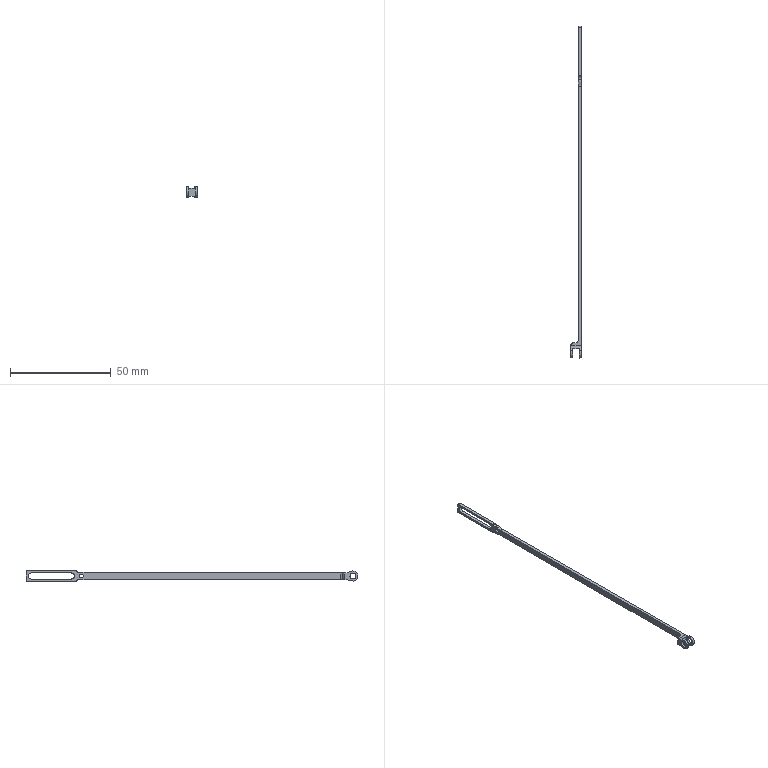Part | STEP file | 2-17 | 1 solid | 35 faces | box 5 x 165 x 5 mm | volume 803.778 mm3 | cylinder 21 | plane 14 | commonest cylinder face diameters 3 x6 1 x4 10 x4 2 x3 4 x2 5 x2